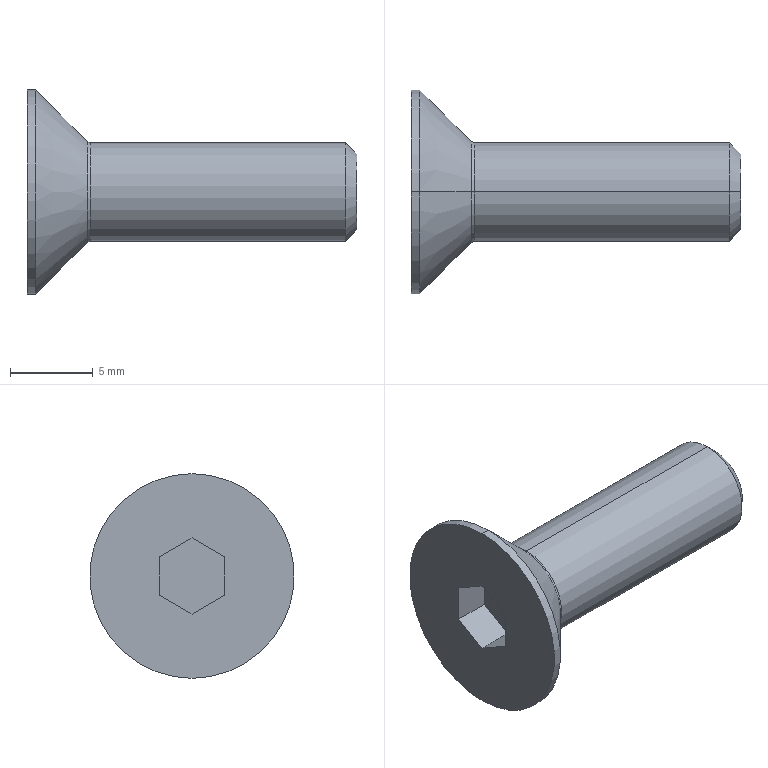Part | STEP file | 1 solid | 19 faces | box 20 x 12.399 x 12.399 mm | volume 709.68 mm3 | plane 9 | cylinder 4 | cone 4 | spline 2 | commonest cylinder face diameters 6 x2 12.399 x2
STEP:
#1=CARTESIAN_POINT('',(0.,0.,0.));
#2=DIRECTION('',(0.,0.,1.));
#3=DIRECTION('',(1.,0.,0.));
#4=AXIS2_PLACEMENT_3D('',#1,#2,#3);
#5=CARTESIAN_POINT('',(-1.52,0.,2.309));
#6=VERTEX_POINT('',#5);
#7=CARTESIAN_POINT('',(-1.52,2.,1.155));
#8=VERTEX_POINT('',#7);
#9=CARTESIAN_POINT('',(-1.52,0.,2.309));
#10=DIRECTION('',(0.,0.866,-0.5));
#11=VECTOR('',#10,1.);
#12=LINE('',#9,#11);
#13=CARTESIAN_POINT('',(-1.52,0.,0.));
#14=DIRECTION('',(-1.,0.,0.));
#15=DIRECTION('',(0.,0.,1.));
#16=AXIS2_PLACEMENT_3D('',#13,#14,#15);
#17=PLANE('',#16);
#18=CARTESIAN_POINT('',(2.309,0.));
#19=DIRECTION('',(-0.5,0.866));
#20=VECTOR('',#19,1.);
#21=LINE('',#18,#20);
#22=(GEOMETRIC_REPRESENTATION_CONTEXT(2)PARAMETRIC_REPRESENTATION_CONTEXT()REPRESENTATION_CONTEXT('',''));
#23=DEFINITIONAL_REPRESENTATION('',(#21),#22);
#24=PCURVE('',#17,#23);
#25=CARTESIAN_POINT('',(-1.52,0.,2.309));
#26=DIRECTION('',(0.,0.5,0.866));
#27=DIRECTION('',(1.,0.,0.));
#28=AXIS2_PLACEMENT_3D('',#25,#26,#27);
#29=PLANE('',#28);
#30=CARTESIAN_POINT('',(0.,0.));
#31=DIRECTION('',(0.,1.));
#32=VECTOR('',#31,1.);
#33=LINE('',#30,#32);
#34=(GEOMETRIC_REPRESENTATION_CONTEXT(2)PARAMETRIC_REPRESENTATION_CONTEXT()REPRESENTATION_CONTEXT('',''));
#35=DEFINITIONAL_REPRESENTATION('',(#33),#34);
#36=PCURVE('',#29,#35);
#37=SURFACE_CURVE('',#12,(#24,#36),.PCURVE_S1.);
#38=EDGE_CURVE('',#6,#8,#37,.T.);
#39=ORIENTED_EDGE('',*,*,#38,.T.);
#40=CARTESIAN_POINT('',(-1.52,2.,-1.155));
#41=VERTEX_POINT('',#40);
#42=CARTESIAN_POINT('',(-1.52,2.,1.155));
#43=DIRECTION('',(0.,0.,-1.));
#44=VECTOR('',#43,1.);
#45=LINE('',#42,#44);
#46=CARTESIAN_POINT('',(1.155,2.));
#47=DIRECTION('',(-1.,0.));
#48=VECTOR('',#47,1.);
#49=LINE('',#46,#48);
#50=(GEOMETRIC_REPRESENTATION_CONTEXT(2)PARAMETRIC_REPRESENTATION_CONTEXT()REPRESENTATION_CONTEXT('',''));
#51=DEFINITIONAL_REPRESENTATION('',(#49),#50);
#52=PCURVE('',#17,#51);
#53=CARTESIAN_POINT('',(-1.52,2.,1.155));
#54=DIRECTION('',(0.,1.,0.));
#55=DIRECTION('',(0.,0.,-1.));
#56=AXIS2_PLACEMENT_3D('',#53,#54,#55);
#57=PLANE('',#56);
#58=CARTESIAN_POINT('',(0.,0.));
#59=DIRECTION('',(1.,0.));
#60=VECTOR('',#59,1.);
#61=LINE('',#58,#60);
#62=(GEOMETRIC_REPRESENTATION_CONTEXT(2)PARAMETRIC_REPRESENTATION_CONTEXT()REPRESENTATION_CONTEXT('',''));
#63=DEFINITIONAL_REPRESENTATION('',(#61),#62);
#64=PCURVE('',#57,#63);
#65=SURFACE_CURVE('',#45,(#52,#64),.PCURVE_S1.);
#66=EDGE_CURVE('',#8,#41,#65,.T.);
#67=ORIENTED_EDGE('',*,*,#66,.T.);
#68=CARTESIAN_POINT('',(-1.52,0.,-2.309));
#69=VERTEX_POINT('',#68);
#70=CARTESIAN_POINT('',(-1.52,2.,-1.155));
#71=DIRECTION('',(0.,-0.866,-0.5));
#72=VECTOR('',#71,1.);
#73=LINE('',#70,#72);
#74=CARTESIAN_POINT('',(-1.155,2.));
#75=DIRECTION('',(-0.5,-0.866));
#76=VECTOR('',#75,1.);
#77=LINE('',#74,#76);
#78=(GEOMETRIC_REPRESENTATION_CONTEXT(2)PARAMETRIC_REPRESENTATION_CONTEXT()REPRESENTATION_CONTEXT('',''));
#79=DEFINITIONAL_REPRESENTATION('',(#77),#78);
#80=PCURVE('',#17,#79);
#81=CARTESIAN_POINT('',(-1.52,2.,-1.155));
#82=DIRECTION('',(0.,0.5,-0.866));
#83=DIRECTION('',(-1.,0.,0.));
#84=AXIS2_PLACEMENT_3D('',#81,#82,#83);
#85=PLANE('',#84);
#86=CARTESIAN_POINT('',(0.,0.));
#87=DIRECTION('',(0.,-1.));
#88=VECTOR('',#87,1.);
#89=LINE('',#86,#88);
#90=(GEOMETRIC_REPRESENTATION_CONTEXT(2)PARAMETRIC_REPRESENTATION_CONTEXT()REPRESENTATION_CONTEXT('',''));
#91=DEFINITIONAL_REPRESENTATION('',(#89),#90);
#92=PCURVE('',#85,#91);
#93=SURFACE_CURVE('',#73,(#80,#92),.PCURVE_S1.);
#94=EDGE_CURVE('',#41,#69,#93,.T.);
#95=ORIENTED_EDGE('',*,*,#94,.T.);
#96=CARTESIAN_POINT('',(-1.52,-2.,-1.155));
#97=VERTEX_POINT('',#96);
#98=CARTESIAN_POINT('',(-1.52,0.,-2.309));
#99=DIRECTION('',(0.,-0.866,0.5));
#100=VECTOR('',#99,1.);
#101=LINE('',#98,#100);
#102=CARTESIAN_POINT('',(-2.309,0.));
#103=DIRECTION('',(0.5,-0.866));
#104=VECTOR('',#103,1.);
#105=LINE('',#102,#104);
#106=(GEOMETRIC_REPRESENTATION_CONTEXT(2)PARAMETRIC_REPRESENTATION_CONTEXT()REPRESENTATION_CONTEXT('',''));
#107=DEFINITIONAL_REPRESENTATION('',(#105),#106);
#108=PCURVE('',#17,#107);
#109=CARTESIAN_POINT('',(-1.52,0.,-2.309));
#110=DIRECTION('',(0.,-0.5,-0.866));
#111=DIRECTION('',(0.,-0.866,0.5));
#112=AXIS2_PLACEMENT_3D('',#109,#110,#111);
#113=PLANE('',#112);
#114=CARTESIAN_POINT('',(0.,0.));
#115=DIRECTION('',(1.,0.));
#116=VECTOR('',#115,1.);
#117=LINE('',#114,#116);
#118=(GEOMETRIC_REPRESENTATION_CONTEXT(2)PARAMETRIC_REPRESENTATION_CONTEXT()REPRESENTATION_CONTEXT('',''));
#119=DEFINITIONAL_REPRESENTATION('',(#117),#118);
#120=PCURVE('',#113,#119);
#121=SURFACE_CURVE('',#101,(#108,#120),.PCURVE_S1.);
#122=EDGE_CURVE('',#69,#97,#121,.T.);
#123=ORIENTED_EDGE('',*,*,#122,.T.);
#124=CARTESIAN_POINT('',(-1.52,-2.,1.155));
#125=VERTEX_POINT('',#124);
#126=CARTESIAN_POINT('',(-1.52,-2.,-1.155));
#127=DIRECTION('',(0.,0.,1.));
#128=VECTOR('',#127,1.);
#129=LINE('',#126,#128);
#130=CARTESIAN_POINT('',(-1.155,-2.));
#131=DIRECTION('',(1.,0.));
#132=VECTOR('',#131,1.);
#133=LINE('',#130,#132);
#134=(GEOMETRIC_REPRESENTATION_CONTEXT(2)PARAMETRIC_REPRESENTATION_CONTEXT()REPRESENTATION_CONTEXT('',''));
#135=DEFINITIONAL_REPRESENTATION('',(#133),#134);
#136=PCURVE('',#17,#135);
#137=CARTESIAN_POINT('',(-1.52,-2.,-1.155));
#138=DIRECTION('',(0.,-1.,0.));
#139=DIRECTION('',(-1.,0.,0.));
#140=AXIS2_PLACEMENT_3D('',#137,#138,#139);
#141=PLANE('',#140);
#142=CARTESIAN_POINT('',(0.,0.));
#143=DIRECTION('',(0.,-1.));
#144=VECTOR('',#143,1.);
#145=LINE('',#142,#144);
#146=(GEOMETRIC_REPRESENTATION_CONTEXT(2)PARAMETRIC_REPRESENTATION_CONTEXT()REPRESENTATION_CONTEXT('',''));
#147=DEFINITIONAL_REPRESENTATION('',(#145),#146);
#148=PCURVE('',#141,#147);
#149=SURFACE_CURVE('',#129,(#136,#148),.PCURVE_S1.);
#150=EDGE_CURVE('',#97,#125,#149,.T.);
#151=ORIENTED_EDGE('',*,*,#150,.T.);
#152=CARTESIAN_POINT('',(-1.52,-2.,1.155));
#153=DIRECTION('',(0.,0.866,0.5));
#154=VECTOR('',#153,1.);
#155=LINE('',#152,#154);
#156=CARTESIAN_POINT('',(1.155,-2.));
#157=DIRECTION('',(0.5,0.866));
#158=VECTOR('',#157,1.);
#159=LINE('',#156,#158);
#160=(GEOMETRIC_REPRESENTATION_CONTEXT(2)PARAMETRIC_REPRESENTATION_CONTEXT()REPRESENTATION_CONTEXT('',''));
#161=DEFINITIONAL_REPRESENTATION('',(#159),#160);
#162=PCURVE('',#17,#161);
#163=CARTESIAN_POINT('',(-1.52,-2.,1.155));
#164=DIRECTION('',(0.,-0.5,0.866));
#165=DIRECTION('',(-1.,0.,0.));
#166=AXIS2_PLACEMENT_3D('',#163,#164,#165);
#167=PLANE('',#166);
#168=CARTESIAN_POINT('',(0.,0.));
#169=DIRECTION('',(0.,-1.));
#170=VECTOR('',#169,1.);
#171=LINE('',#168,#170);
#172=(GEOMETRIC_REPRESENTATION_CONTEXT(2)PARAMETRIC_REPRESENTATION_CONTEXT()REPRESENTATION_CONTEXT('',''));
#173=DEFINITIONAL_REPRESENTATION('',(#171),#172);
#174=PCURVE('',#167,#173);
#175=SURFACE_CURVE('',#155,(#162,#174),.PCURVE_S1.);
#176=EDGE_CURVE('',#125,#6,#175,.T.);
#177=ORIENTED_EDGE('',*,*,#176,.T.);
#178=EDGE_LOOP('',(#39,#67,#95,#123,#151,#177));
#179=FACE_BOUND('',#178,.T.);
#180=ADVANCED_FACE('',(#179),#17,.T.);
#181=CARTESIAN_POINT('',(-3.72,0.,-2.309));
#182=VERTEX_POINT('',#181);
#183=CARTESIAN_POINT('',(-1.52,0.,-2.309));
#184=DIRECTION('',(1.,0.,0.));
#185=VECTOR('',#184,1.);
#186=LINE('',#183,#185);
#187=CARTESIAN_POINT('',(0.,-2.309));
#188=DIRECTION('',(-1.,0.));
#189=VECTOR('',#188,1.);
#190=LINE('',#187,#189);
#191=(GEOMETRIC_REPRESENTATION_CONTEXT(2)PARAMETRIC_REPRESENTATION_CONTEXT()REPRESENTATION_CONTEXT('',''));
#192=DEFINITIONAL_REPRESENTATION('',(#190),#191);
#193=PCURVE('',#85,#192);
#194=CARTESIAN_POINT('',(0.,0.));
#195=DIRECTION('',(0.,-1.));
#196=VECTOR('',#195,1.);
#197=LINE('',#194,#196);
#198=(GEOMETRIC_REPRESENTATION_CONTEXT(2)PARAMETRIC_REPRESENTATION_CONTEXT()REPRESENTATION_CONTEXT('',''));
#199=DEFINITIONAL_REPRESENTATION('',(#197),#198);
#200=PCURVE('',#113,#199);
#201=SURFACE_CURVE('',#186,(#193,#200),.PCURVE_S1.);
#202=EDGE_CURVE('',#182,#69,#201,.T.);
#203=ORIENTED_EDGE('',*,*,#202,.T.);
#204=ORIENTED_EDGE('',*,*,#94,.F.);
#205=CARTESIAN_POINT('',(-3.72,2.,-1.155));
#206=VERTEX_POINT('',#205);
#207=CARTESIAN_POINT('',(-1.52,2.,-1.155));
#208=DIRECTION('',(-1.,0.,0.));
#209=VECTOR('',#208,1.);
#210=LINE('',#207,#209);
#211=CARTESIAN_POINT('',(0.,0.));
#212=DIRECTION('',(1.,0.));
#213=VECTOR('',#212,1.);
#214=LINE('',#211,#213);
#215=(GEOMETRIC_REPRESENTATION_CONTEXT(2)PARAMETRIC_REPRESENTATION_CONTEXT()REPRESENTATION_CONTEXT('',''));
#216=DEFINITIONAL_REPRESENTATION('',(#214),#215);
#217=PCURVE('',#85,#216);
#218=CARTESIAN_POINT('',(2.309,0.));
#219=DIRECTION('',(0.,1.));
#220=VECTOR('',#219,1.);
#221=LINE('',#218,#220);
#222=(GEOMETRIC_REPRESENTATION_CONTEXT(2)PARAMETRIC_REPRESENTATION_CONTEXT()REPRESENTATION_CONTEXT('',''));
#223=DEFINITIONAL_REPRESENTATION('',(#221),#222);
#224=PCURVE('',#57,#223);
#225=SURFACE_CURVE('',#210,(#217,#224),.PCURVE_S1.);
#226=EDGE_CURVE('',#41,#206,#225,.T.);
#227=ORIENTED_EDGE('',*,*,#226,.T.);
#228=CARTESIAN_POINT('',(-3.72,0.,-2.309));
#229=DIRECTION('',(0.,0.866,0.5));
#230=VECTOR('',#229,1.);
#231=LINE('',#228,#230);
#232=CARTESIAN_POINT('',(2.2,-2.309));
#233=DIRECTION('',(0.,1.));
#234=VECTOR('',#233,1.);
#235=LINE('',#232,#234);
#236=(GEOMETRIC_REPRESENTATION_CONTEXT(2)PARAMETRIC_REPRESENTATION_CONTEXT()REPRESENTATION_CONTEXT('',''));
#237=DEFINITIONAL_REPRESENTATION('',(#235),#236);
#238=PCURVE('',#85,#237);
#239=CARTESIAN_POINT('',(-3.72,0.,0.));
#240=DIRECTION('',(-1.,0.,0.));
#241=DIRECTION('',(0.,0.,1.));
#242=AXIS2_PLACEMENT_3D('',#239,#240,#241);
#243=PLANE('',#242);
#244=CARTESIAN_POINT('',(-2.309,0.));
#245=DIRECTION('',(0.5,0.866));
#246=VECTOR('',#245,1.);
#247=LINE('',#244,#246);
#248=(GEOMETRIC_REPRESENTATION_CONTEXT(2)PARAMETRIC_REPRESENTATION_CONTEXT()REPRESENTATION_CONTEXT('',''));
#249=DEFINITIONAL_REPRESENTATION('',(#247),#248);
#250=PCURVE('',#243,#249);
#251=SURFACE_CURVE('',#231,(#238,#250),.PCURVE_S1.);
#252=EDGE_CURVE('',#182,#206,#251,.T.);
#253=ORIENTED_EDGE('',*,*,#252,.F.);
#254=EDGE_LOOP('',(#203,#204,#227,#253));
#255=FACE_BOUND('',#254,.T.);
#256=ADVANCED_FACE('',(#255),#85,.F.);
#257=ORIENTED_EDGE('',*,*,#226,.F.);
#258=ORIENTED_EDGE('',*,*,#66,.F.);
#259=CARTESIAN_POINT('',(-3.72,2.,1.155));
#260=VERTEX_POINT('',#259);
#261=CARTESIAN_POINT('',(-1.52,2.,1.155));
#262=DIRECTION('',(-1.,0.,0.));
#263=VECTOR('',#262,1.);
#264=LINE('',#261,#263);
#265=CARTESIAN_POINT('',(0.,0.));
#266=DIRECTION('',(0.,1.));
#267=VECTOR('',#266,1.);
#268=LINE('',#265,#267);
#269=(GEOMETRIC_REPRESENTATION_CONTEXT(2)PARAMETRIC_REPRESENTATION_CONTEXT()REPRESENTATION_CONTEXT('',''));
#270=DEFINITIONAL_REPRESENTATION('',(#268),#269);
#271=PCURVE('',#57,#270);
#272=CARTESIAN_POINT('',(0.,2.309));
#273=DIRECTION('',(-1.,0.));
#274=VECTOR('',#273,1.);
#275=LINE('',#272,#274);
#276=(GEOMETRIC_REPRESENTATION_CONTEXT(2)PARAMETRIC_REPRESENTATION_CONTEXT()REPRESENTATION_CONTEXT('',''));
#277=DEFINITIONAL_REPRESENTATION('',(#275),#276);
#278=PCURVE('',#29,#277);
#279=SURFACE_CURVE('',#264,(#271,#278),.PCURVE_S1.);
#280=EDGE_CURVE('',#8,#260,#279,.T.);
#281=ORIENTED_EDGE('',*,*,#280,.T.);
#282=CARTESIAN_POINT('',(-3.72,2.,0.));
#283=DIRECTION('',(0.,0.,1.));
#284=VECTOR('',#283,1.);
#285=LINE('',#282,#284);
#286=CARTESIAN_POINT('',(1.155,2.2));
#287=DIRECTION('',(-1.,0.));
#288=VECTOR('',#287,1.);
#289=LINE('',#286,#288);
#290=(GEOMETRIC_REPRESENTATION_CONTEXT(2)PARAMETRIC_REPRESENTATION_CONTEXT()REPRESENTATION_CONTEXT('',''));
#291=DEFINITIONAL_REPRESENTATION('',(#289),#290);
#292=PCURVE('',#57,#291);
#293=CARTESIAN_POINT('',(0.,2.));
#294=DIRECTION('',(1.,0.));
#295=VECTOR('',#294,1.);
#296=LINE('',#293,#295);
#297=(GEOMETRIC_REPRESENTATION_CONTEXT(2)PARAMETRIC_REPRESENTATION_CONTEXT()REPRESENTATION_CONTEXT('',''));
#298=DEFINITIONAL_REPRESENTATION('',(#296),#297);
#299=PCURVE('',#243,#298);
#300=SURFACE_CURVE('',#285,(#292,#299),.PCURVE_S1.);
#301=EDGE_CURVE('',#206,#260,#300,.T.);
#302=ORIENTED_EDGE('',*,*,#301,.F.);
#303=EDGE_LOOP('',(#257,#258,#281,#302));
#304=FACE_BOUND('',#303,.T.);
#305=ADVANCED_FACE('',(#304),#57,.F.);
#306=ORIENTED_EDGE('',*,*,#280,.F.);
#307=ORIENTED_EDGE('',*,*,#38,.F.);
#308=CARTESIAN_POINT('',(-3.72,0.,2.309));
#309=VERTEX_POINT('',#308);
#310=CARTESIAN_POINT('',(-1.52,0.,2.309));
#311=DIRECTION('',(-1.,0.,0.));
#312=VECTOR('',#311,1.);
#313=LINE('',#310,#312);
#314=CARTESIAN_POINT('',(0.,0.));
#315=DIRECTION('',(-1.,0.));
#316=VECTOR('',#315,1.);
#317=LINE('',#314,#316);
#318=(GEOMETRIC_REPRESENTATION_CONTEXT(2)PARAMETRIC_REPRESENTATION_CONTEXT()REPRESENTATION_CONTEXT('',''));
#319=DEFINITIONAL_REPRESENTATION('',(#317),#318);
#320=PCURVE('',#29,#319);
#321=CARTESIAN_POINT('',(0.,-2.309));
#322=DIRECTION('',(1.,0.));
#323=VECTOR('',#322,1.);
#324=LINE('',#321,#323);
#325=(GEOMETRIC_REPRESENTATION_CONTEXT(2)PARAMETRIC_REPRESENTATION_CONTEXT()REPRESENTATION_CONTEXT('',''));
#326=DEFINITIONAL_REPRESENTATION('',(#324),#325);
#327=PCURVE('',#167,#326);
#328=SURFACE_CURVE('',#313,(#320,#327),.PCURVE_S1.);
#329=EDGE_CURVE('',#6,#309,#328,.T.);
#330=ORIENTED_EDGE('',*,*,#329,.T.);
#331=CARTESIAN_POINT('',(-3.72,2.,1.155));
#332=DIRECTION('',(0.,-0.866,0.5));
#333=VECTOR('',#332,1.);
#334=LINE('',#331,#333);
#335=CARTESIAN_POINT('',(-2.2,2.309));
#336=DIRECTION('',(0.,-1.));
#337=VECTOR('',#336,1.);
#338=LINE('',#335,#337);
#339=(GEOMETRIC_REPRESENTATION_CONTEXT(2)PARAMETRIC_REPRESENTATION_CONTEXT()REPRESENTATION_CONTEXT('',''));
#340=DEFINITIONAL_REPRESENTATION('',(#338),#339);
#341=PCURVE('',#29,#340);
#342=CARTESIAN_POINT('',(1.155,2.));
#343=DIRECTION('',(0.5,-0.866));
#344=VECTOR('',#343,1.);
#345=LINE('',#342,#344);
#346=(GEOMETRIC_REPRESENTATION_CONTEXT(2)PARAMETRIC_REPRESENTATION_CONTEXT()REPRESENTATION_CONTEXT('',''));
#347=DEFINITIONAL_REPRESENTATION('',(#345),#346);
#348=PCURVE('',#243,#347);
#349=SURFACE_CURVE('',#334,(#341,#348),.PCURVE_S1.);
#350=EDGE_CURVE('',#260,#309,#349,.T.);
#351=ORIENTED_EDGE('',*,*,#350,.F.);
#352=EDGE_LOOP('',(#306,#307,#330,#351));
#353=FACE_BOUND('',#352,.T.);
#354=ADVANCED_FACE('',(#353),#29,.F.);
#355=ORIENTED_EDGE('',*,*,#329,.F.);
#356=ORIENTED_EDGE('',*,*,#176,.F.);
#357=CARTESIAN_POINT('',(-3.72,-2.,1.155));
#358=VERTEX_POINT('',#357);
#359=CARTESIAN_POINT('',(-1.52,-2.,1.155));
#360=DIRECTION('',(-1.,0.,0.));
#361=VECTOR('',#360,1.);
#362=LINE('',#359,#361);
#363=CARTESIAN_POINT('',(0.,0.));
#364=DIRECTION('',(1.,0.));
#365=VECTOR('',#364,1.);
#366=LINE('',#363,#365);
#367=(GEOMETRIC_REPRESENTATION_CONTEXT(2)PARAMETRIC_REPRESENTATION_CONTEXT()REPRESENTATION_CONTEXT('',''));
#368=DEFINITIONAL_REPRESENTATION('',(#366),#367);
#369=PCURVE('',#167,#368);
#370=CARTESIAN_POINT('',(0.,-2.309));
#371=DIRECTION('',(1.,0.));
#372=VECTOR('',#371,1.);
#373=LINE('',#370,#372);
#374=(GEOMETRIC_REPRESENTATION_CONTEXT(2)PARAMETRIC_REPRESENTATION_CONTEXT()REPRESENTATION_CONTEXT('',''));
#375=DEFINITIONAL_REPRESENTATION('',(#373),#374);
#376=PCURVE('',#141,#375);
#377=SURFACE_CURVE('',#362,(#369,#376),.PCURVE_S1.);
#378=EDGE_CURVE('',#125,#358,#377,.T.);
#379=ORIENTED_EDGE('',*,*,#378,.T.);
#380=CARTESIAN_POINT('',(-3.72,0.,2.309));
#381=DIRECTION('',(0.,-0.866,-0.5));
#382=VECTOR('',#381,1.);
#383=LINE('',#380,#382);
#384=CARTESIAN_POINT('',(2.2,-2.309));
#385=DIRECTION('',(0.,1.));
#386=VECTOR('',#385,1.);
#387=LINE('',#384,#386);
#388=(GEOMETRIC_REPRESENTATION_CONTEXT(2)PARAMETRIC_REPRESENTATION_CONTEXT()REPRESENTATION_CONTEXT('',''));
#389=DEFINITIONAL_REPRESENTATION('',(#387),#388);
#390=PCURVE('',#167,#389);
#391=CARTESIAN_POINT('',(2.309,0.));
#392=DIRECTION('',(-0.5,-0.866));
#393=VECTOR('',#392,1.);
#394=LINE('',#391,#393);
#395=(GEOMETRIC_REPRESENTATION_CONTEXT(2)PARAMETRIC_REPRESENTATION_CONTEXT()REPRESENTATION_CONTEXT('',''));
#396=DEFINITIONAL_REPRESENTATION('',(#394),#395);
#397=PCURVE('',#243,#396);
#398=SURFACE_CURVE('',#383,(#390,#397),.PCURVE_S1.);
#399=EDGE_CURVE('',#309,#358,#398,.T.);
#400=ORIENTED_EDGE('',*,*,#399,.F.);
#401=EDGE_LOOP('',(#355,#356,#379,#400));
#402=FACE_BOUND('',#401,.T.);
#403=ADVANCED_FACE('',(#402),#167,.F.);
#404=ORIENTED_EDGE('',*,*,#378,.F.);
#405=ORIENTED_EDGE('',*,*,#150,.F.);
#406=CARTESIAN_POINT('',(-3.72,-2.,-1.155));
#407=VERTEX_POINT('',#406);
#408=CARTESIAN_POINT('',(-1.52,-2.,-1.155));
#409=DIRECTION('',(-1.,0.,0.));
#410=VECTOR('',#409,1.);
#411=LINE('',#408,#410);
#412=CARTESIAN_POINT('',(0.,0.));
#413=DIRECTION('',(1.,0.));
#414=VECTOR('',#413,1.);
#415=LINE('',#412,#414);
#416=(GEOMETRIC_REPRESENTATION_CONTEXT(2)PARAMETRIC_REPRESENTATION_CONTEXT()REPRESENTATION_CONTEXT('',''));
#417=DEFINITIONAL_REPRESENTATION('',(#415),#416);
#418=PCURVE('',#141,#417);
#419=CARTESIAN_POINT('',(2.309,0.));
#420=DIRECTION('',(0.,1.));
#421=VECTOR('',#420,1.);
#422=LINE('',#419,#421);
#423=(GEOMETRIC_REPRESENTATION_CONTEXT(2)PARAMETRIC_REPRESENTATION_CONTEXT()REPRESENTATION_CONTEXT('',''));
#424=DEFINITIONAL_REPRESENTATION('',(#422),#423);
#425=PCURVE('',#113,#424);
#426=SURFACE_CURVE('',#411,(#418,#425),.PCURVE_S1.);
#427=EDGE_CURVE('',#97,#407,#426,.T.);
#428=ORIENTED_EDGE('',*,*,#427,.T.);
#429=CARTESIAN_POINT('',(-3.72,-2.,0.));
#430=DIRECTION('',(0.,0.,-1.));
#431=VECTOR('',#430,1.);
#432=LINE('',#429,#431);
#433=CARTESIAN_POINT('',(2.2,-1.155));
#434=DIRECTION('',(0.,1.));
#435=VECTOR('',#434,1.);
#436=LINE('',#433,#435);
#437=(GEOMETRIC_REPRESENTATION_CONTEXT(2)PARAMETRIC_REPRESENTATION_CONTEXT()REPRESENTATION_CONTEXT('',''));
#438=DEFINITIONAL_REPRESENTATION('',(#436),#437);
#439=PCURVE('',#141,#438);
#440=CARTESIAN_POINT('',(0.,-2.));
#441=DIRECTION('',(-1.,0.));
#442=VECTOR('',#441,1.);
#443=LINE('',#440,#442);
#444=(GEOMETRIC_REPRESENTATION_CONTEXT(2)PARAMETRIC_REPRESENTATION_CONTEXT()REPRESENTATION_CONTEXT('',''));
#445=DEFINITIONAL_REPRESENTATION('',(#443),#444);
#446=PCURVE('',#243,#445);
#447=SURFACE_CURVE('',#432,(#439,#446),.PCURVE_S1.);
#448=EDGE_CURVE('',#358,#407,#447,.T.);
#449=ORIENTED_EDGE('',*,*,#448,.F.);
#450=EDGE_LOOP('',(#404,#405,#428,#449));
#451=FACE_BOUND('',#450,.T.);
#452=ADVANCED_FACE('',(#451),#141,.F.);
#453=ORIENTED_EDGE('',*,*,#427,.F.);
#454=ORIENTED_EDGE('',*,*,#122,.F.);
#455=ORIENTED_EDGE('',*,*,#202,.F.);
#456=CARTESIAN_POINT('',(-3.72,-2.,-1.155));
#457=DIRECTION('',(0.,0.866,-0.5));
#458=VECTOR('',#457,1.);
#459=LINE('',#456,#458);
#460=CARTESIAN_POINT('',(2.309,2.2));
#461=DIRECTION('',(-1.,0.));
#462=VECTOR('',#461,1.);
#463=LINE('',#460,#462);
#464=(GEOMETRIC_REPRESENTATION_CONTEXT(2)PARAMETRIC_REPRESENTATION_CONTEXT()REPRESENTATION_CONTEXT('',''));
#465=DEFINITIONAL_REPRESENTATION('',(#463),#464);
#466=PCURVE('',#113,#465);
#467=CARTESIAN_POINT('',(-1.155,-2.));
#468=DIRECTION('',(-0.5,0.866));
#469=VECTOR('',#468,1.);
#470=LINE('',#467,#469);
#471=(GEOMETRIC_REPRESENTATION_CONTEXT(2)PARAMETRIC_REPRESENTATION_CONTEXT()REPRESENTATION_CONTEXT('',''));
#472=DEFINITIONAL_REPRESENTATION('',(#470),#471);
#473=PCURVE('',#243,#472);
#474=SURFACE_CURVE('',#459,(#466,#473),.PCURVE_S1.);
#475=EDGE_CURVE('',#407,#182,#474,.T.);
#476=ORIENTED_EDGE('',*,*,#475,.F.);
#477=EDGE_LOOP('',(#453,#454,#455,#476));
#478=FACE_BOUND('',#477,.T.);
#479=ADVANCED_FACE('',(#478),#113,.F.);
#480=ORIENTED_EDGE('',*,*,#448,.T.);
#481=ORIENTED_EDGE('',*,*,#475,.T.);
#482=ORIENTED_EDGE('',*,*,#252,.T.);
#483=ORIENTED_EDGE('',*,*,#301,.T.);
#484=ORIENTED_EDGE('',*,*,#350,.T.);
#485=ORIENTED_EDGE('',*,*,#399,.T.);
#486=EDGE_LOOP('',(#480,#481,#482,#483,#484,#485));
#487=FACE_BOUND('',#486,.T.);
#488=CARTESIAN_POINT('',(-3.72,0.,6.2));
#489=VERTEX_POINT('',#488);
#490=CARTESIAN_POINT('',(-3.72,0.,-6.2));
#491=VERTEX_POINT('',#490);
#492=CARTESIAN_POINT('',(-3.72,0.,0.));
#493=DIRECTION('',(1.,0.,0.));
#494=DIRECTION('',(0.,0.,1.));
#495=AXIS2_PLACEMENT_3D('',#492,#493,#494);
#496=CIRCLE('',#495,6.2);
#497=CARTESIAN_POINT('',(6.2,0.));
#498=CARTESIAN_POINT('',(6.2,-10.738));
#499=CARTESIAN_POINT('',(-3.1,-5.369));
#500=CARTESIAN_POINT('',(-12.399,0.));
#501=CARTESIAN_POINT('',(-3.1,5.369));
#502=CARTESIAN_POINT('',(6.2,10.738));
#503=CARTESIAN_POINT('',(6.2,0.));
#504=(BOUNDED_CURVE()B_SPLINE_CURVE(2,(#497,#498,#499,#500,#501,#502,#503),.UNSPECIFIED.,.T.,.F.)B_SPLINE_CURVE_WITH_KNOTS((1,2,2,2,2,1),(-2.094,0.,2.094,4.189,6.283,8.378),.UNSPECIFIED.)CURVE()GEOMETRIC_REPRESENTATION_ITEM()RATIONAL_B_SPLINE_CURVE((1.,0.5,1.,0.5,1.,0.5,1.))REPRESENTATION_ITEM(''));
#505=(GEOMETRIC_REPRESENTATION_CONTEXT(2)PARAMETRIC_REPRESENTATION_CONTEXT()REPRESENTATION_CONTEXT('',''));
#506=DEFINITIONAL_REPRESENTATION('',(#504),#505);
#507=PCURVE('',#243,#506);
#508=CARTESIAN_POINT('',(16.28,0.,0.));
#509=DIRECTION('',(-1.,0.,0.));
#510=DIRECTION('',(0.,0.,1.));
#511=AXIS2_PLACEMENT_3D('',#508,#509,#510);
#512=CYLINDRICAL_SURFACE('',#511,6.2);
#513=CARTESIAN_POINT('',(6.283,20.));
#514=DIRECTION('',(-1.,0.));
#515=VECTOR('',#514,1.);
#516=LINE('',#513,#515);
#517=(GEOMETRIC_REPRESENTATION_CONTEXT(2)PARAMETRIC_REPRESENTATION_CONTEXT()REPRESENTATION_CONTEXT('',''));
#518=DEFINITIONAL_REPRESENTATION('',(#516),#517);
#519=PCURVE('',#512,#518);
#520=SURFACE_CURVE('',#496,(#507,#519),.PCURVE_S1.);
#521=EDGE_CURVE('',#489,#491,#520,.T.);
#522=ORIENTED_EDGE('',*,*,#521,.F.);
#523=CARTESIAN_POINT('',(-3.72,0.,0.));
#524=DIRECTION('',(1.,0.,0.));
#525=DIRECTION('',(0.,0.,1.));
#526=AXIS2_PLACEMENT_3D('',#523,#524,#525);
#527=CIRCLE('',#526,6.2);
#528=CARTESIAN_POINT('',(6.2,0.));
#529=CARTESIAN_POINT('',(6.2,-10.738));
#530=CARTESIAN_POINT('',(-3.1,-5.369));
#531=CARTESIAN_POINT('',(-12.399,0.));
#532=CARTESIAN_POINT('',(-3.1,5.369));
#533=CARTESIAN_POINT('',(6.2,10.738));
#534=CARTESIAN_POINT('',(6.2,0.));
#535=(BOUNDED_CURVE()B_SPLINE_CURVE(2,(#528,#529,#530,#531,#532,#533,#534),.UNSPECIFIED.,.T.,.F.)B_SPLINE_CURVE_WITH_KNOTS((1,2,2,2,2,1),(-2.094,0.,2.094,4.189,6.283,8.378),.UNSPECIFIED.)CURVE()GEOMETRIC_REPRESENTATION_ITEM()RATIONAL_B_SPLINE_CURVE((1.,0.5,1.,0.5,1.,0.5,1.))REPRESENTATION_ITEM(''));
#536=(GEOMETRIC_REPRESENTATION_CONTEXT(2)PARAMETRIC_REPRESENTATION_CONTEXT()REPRESENTATION_CONTEXT('',''));
#537=DEFINITIONAL_REPRESENTATION('',(#535),#536);
#538=PCURVE('',#243,#537);
#539=CARTESIAN_POINT('',(16.28,0.,0.));
#540=DIRECTION('',(-1.,0.,0.));
#541=DIRECTION('',(0.,0.,1.));
#542=AXIS2_PLACEMENT_3D('',#539,#540,#541);
#543=CYLINDRICAL_SURFACE('',#542,6.2);
#544=CARTESIAN_POINT('',(6.283,20.));
#545=DIRECTION('',(-1.,0.));
#546=VECTOR('',#545,1.);
#547=LINE('',#544,#546);
#548=(GEOMETRIC_REPRESENTATION_CONTEXT(2)PARAMETRIC_REPRESENTATION_CONTEXT()REPRESENTATION_CONTEXT('',''));
#549=DEFINITIONAL_REPRESENTATION('',(#547),#548);
#550=PCURVE('',#543,#549);
#551=SURFACE_CURVE('',#527,(#538,#550),.PCURVE_S1.);
#552=EDGE_CURVE('',#491,#489,#551,.T.);
#553=ORIENTED_EDGE('',*,*,#552,.F.);
#554=EDGE_LOOP('',(#522,#553));
#555=FACE_BOUND('',#554,.T.);
#556=ADVANCED_FACE('',(#487,#555),#243,.T.);
#557=CARTESIAN_POINT('',(-3.2,0.,-6.2));
#558=VERTEX_POINT('',#557);
#559=CARTESIAN_POINT('',(16.28,0.,-6.2));
#560=DIRECTION('',(-1.,0.,0.));
#561=VECTOR('',#560,1.);
#562=LINE('',#559,#561);
#563=CARTESIAN_POINT('',(3.142,0.));
#564=DIRECTION('',(0.,1.));
#565=VECTOR('',#564,1.);
#566=LINE('',#563,#565);
#567=(GEOMETRIC_REPRESENTATION_CONTEXT(2)PARAMETRIC_REPRESENTATION_CONTEXT()REPRESENTATION_CONTEXT('',''));
#568=DEFINITIONAL_REPRESENTATION('',(#566),#567);
#569=PCURVE('',#512,#568);
#570=CARTESIAN_POINT('',(3.142,0.));
#571=DIRECTION('',(0.,1.));
#572=VECTOR('',#571,1.);
#573=LINE('',#570,#572);
#574=(GEOMETRIC_REPRESENTATION_CONTEXT(2)PARAMETRIC_REPRESENTATION_CONTEXT()REPRESENTATION_CONTEXT('',''));
#575=DEFINITIONAL_REPRESENTATION('',(#573),#574);
#576=PCURVE('',#543,#575);
#577=SURFACE_CURVE('',#562,(#569,#576),.PCURVE_S1.);
#578=EDGE_CURVE('',#558,#491,#577,.T.);
#579=ORIENTED_EDGE('',*,*,#578,.F.);
#580=CARTESIAN_POINT('',(-3.2,0.,6.2));
#581=VERTEX_POINT('',#580);
#582=CARTESIAN_POINT('',(-3.2,0.,0.));
#583=DIRECTION('',(1.,0.,0.));
#584=DIRECTION('',(0.,0.,1.));
#585=AXIS2_PLACEMENT_3D('',#582,#583,#584);
#586=CIRCLE('',#585,6.2);
#587=CARTESIAN_POINT('',(6.283,19.48));
#588=DIRECTION('',(-1.,0.));
#589=VECTOR('',#588,1.);
#590=LINE('',#587,#589);
#591=(GEOMETRIC_REPRESENTATION_CONTEXT(2)PARAMETRIC_REPRESENTATION_CONTEXT()REPRESENTATION_CONTEXT('',''));
#592=DEFINITIONAL_REPRESENTATION('',(#590),#591);
#593=PCURVE('',#512,#592);
#594=CARTESIAN_POINT('',(-3.2,0.,0.));
#595=DIRECTION('',(-1.,0.,0.));
#596=DIRECTION('',(0.,0.,1.));
#597=AXIS2_PLACEMENT_3D('',#594,#595,#596);
#598=CONICAL_SURFACE('',#597,6.2,0.7854);
#599=CARTESIAN_POINT('',(6.283,0.));
#600=DIRECTION('',(-1.,0.));
#601=VECTOR('',#600,1.);
#602=LINE('',#599,#601);
#603=(GEOMETRIC_REPRESENTATION_CONTEXT(2)PARAMETRIC_REPRESENTATION_CONTEXT()REPRESENTATION_CONTEXT('',''));
#604=DEFINITIONAL_REPRESENTATION('',(#602),#603);
#605=PCURVE('',#598,#604);
#606=SURFACE_CURVE('',#586,(#593,#605),.PCURVE_S1.);
#607=EDGE_CURVE('',#581,#558,#606,.T.);
#608=ORIENTED_EDGE('',*,*,#607,.F.);
#609=CARTESIAN_POINT('',(16.28,0.,6.2));
#610=DIRECTION('',(-1.,0.,0.));
#611=VECTOR('',#610,1.);
#612=LINE('',#609,#611);
#613=CARTESIAN_POINT('',(6.283,0.));
#614=DIRECTION('',(0.,1.));
#615=VECTOR('',#614,1.);
#616=LINE('',#613,#615);
#617=(GEOMETRIC_REPRESENTATION_CONTEXT(2)PARAMETRIC_REPRESENTATION_CONTEXT()REPRESENTATION_CONTEXT('',''));
#618=DEFINITIONAL_REPRESENTATION('',(#616),#617);
#619=PCURVE('',#512,#618);
#620=CARTESIAN_POINT('',(0.,0.));
#621=DIRECTION('',(0.,1.));
#622=VECTOR('',#621,1.);
#623=LINE('',#620,#622);
#624=(GEOMETRIC_REPRESENTATION_CONTEXT(2)PARAMETRIC_REPRESENTATION_CONTEXT()REPRESENTATION_CONTEXT('',''));
#625=DEFINITIONAL_REPRESENTATION('',(#623),#624);
#626=PCURVE('',#543,#625);
#627=SURFACE_CURVE('',#612,(#619,#626),.PCURVE_S1.);
#628=EDGE_CURVE('',#581,#489,#627,.T.);
#629=ORIENTED_EDGE('',*,*,#628,.T.);
#630=ORIENTED_EDGE('',*,*,#521,.T.);
#631=EDGE_LOOP('',(#579,#608,#629,#630));
#632=FACE_BOUND('',#631,.T.);
#633=ADVANCED_FACE('',(#632),#512,.T.);
#634=CARTESIAN_POINT('',(16.28,0.,2.3));
#635=VERTEX_POINT('',#634);
#636=CARTESIAN_POINT('',(16.28,0.,-2.3));
#637=VERTEX_POINT('',#636);
#638=CARTESIAN_POINT('',(16.28,0.,0.));
#639=DIRECTION('',(-1.,0.,0.));
#640=DIRECTION('',(0.,0.,1.));
#641=AXIS2_PLACEMENT_3D('',#638,#639,#640);
#642=CIRCLE('',#641,2.3);
#643=CARTESIAN_POINT('',(16.28,3.,0.));
#644=DIRECTION('',(1.,0.,0.));
#645=DIRECTION('',(0.,1.,0.));
#646=AXIS2_PLACEMENT_3D('',#643,#644,#645);
#647=PLANE('',#646);
#648=CARTESIAN_POINT('',(-3.,2.3));
#649=CARTESIAN_POINT('',(0.9837,2.3));
#650=CARTESIAN_POINT('',(-1.008,-1.15));
#651=CARTESIAN_POINT('',(-3.,-4.6));
#652=CARTESIAN_POINT('',(-4.992,-1.15));
#653=CARTESIAN_POINT('',(-6.984,2.3));
#654=CARTESIAN_POINT('',(-3.,2.3));
#655=(BOUNDED_CURVE()B_SPLINE_CURVE(2,(#648,#649,#650,#651,#652,#653,#654),.UNSPECIFIED.,.T.,.F.)B_SPLINE_CURVE_WITH_KNOTS((1,2,2,2,2,1),(-2.094,0.,2.094,4.189,6.283,8.378),.UNSPECIFIED.)CURVE()GEOMETRIC_REPRESENTATION_ITEM()RATIONAL_B_SPLINE_CURVE((1.,0.5,1.,0.5,1.,0.5,1.))REPRESENTATION_ITEM(''));
#656=(GEOMETRIC_REPRESENTATION_CONTEXT(2)PARAMETRIC_REPRESENTATION_CONTEXT()REPRESENTATION_CONTEXT('',''));
#657=DEFINITIONAL_REPRESENTATION('',(#655),#656);
#658=PCURVE('',#647,#657);
#659=CARTESIAN_POINT('',(15.58,0.,0.));
#660=DIRECTION('',(-1.,0.,0.));
#661=DIRECTION('',(0.,0.,1.));
#662=AXIS2_PLACEMENT_3D('',#659,#660,#661);
#663=CONICAL_SURFACE('',#662,3.,0.7854);
#664=CARTESIAN_POINT('',(0.,-0.7));
#665=DIRECTION('',(1.,0.));
#666=VECTOR('',#665,1.);
#667=LINE('',#664,#666);
#668=(GEOMETRIC_REPRESENTATION_CONTEXT(2)PARAMETRIC_REPRESENTATION_CONTEXT()REPRESENTATION_CONTEXT('',''));
#669=DEFINITIONAL_REPRESENTATION('',(#667),#668);
#670=PCURVE('',#663,#669);
#671=SURFACE_CURVE('',#642,(#658,#670),.PCURVE_S1.);
#672=EDGE_CURVE('',#635,#637,#671,.T.);
#673=ORIENTED_EDGE('',*,*,#672,.F.);
#674=CARTESIAN_POINT('',(16.28,0.,0.));
#675=DIRECTION('',(-1.,0.,0.));
#676=DIRECTION('',(0.,0.,1.));
#677=AXIS2_PLACEMENT_3D('',#674,#675,#676);
#678=CIRCLE('',#677,2.3);
#679=CARTESIAN_POINT('',(-3.,2.3));
#680=CARTESIAN_POINT('',(0.9837,2.3));
#681=CARTESIAN_POINT('',(-1.008,-1.15));
#682=CARTESIAN_POINT('',(-3.,-4.6));
#683=CARTESIAN_POINT('',(-4.992,-1.15));
#684=CARTESIAN_POINT('',(-6.984,2.3));
#685=CARTESIAN_POINT('',(-3.,2.3));
#686=(BOUNDED_CURVE()B_SPLINE_CURVE(2,(#679,#680,#681,#682,#683,#684,#685),.UNSPECIFIED.,.T.,.F.)B_SPLINE_CURVE_WITH_KNOTS((1,2,2,2,2,1),(-2.094,0.,2.094,4.189,6.283,8.378),.UNSPECIFIED.)CURVE()GEOMETRIC_REPRESENTATION_ITEM()RATIONAL_B_SPLINE_CURVE((1.,0.5,1.,0.5,1.,0.5,1.))REPRESENTATION_ITEM(''));
#687=(GEOMETRIC_REPRESENTATION_CONTEXT(2)PARAMETRIC_REPRESENTATION_CONTEXT()REPRESENTATION_CONTEXT('',''));
#688=DEFINITIONAL_REPRESENTATION('',(#686),#687);
#689=PCURVE('',#647,#688);
#690=CARTESIAN_POINT('',(15.58,0.,0.));
#691=DIRECTION('',(-1.,0.,0.));
#692=DIRECTION('',(0.,0.,1.));
#693=AXIS2_PLACEMENT_3D('',#690,#691,#692);
#694=CONICAL_SURFACE('',#693,3.,0.7854);
#695=CARTESIAN_POINT('',(0.,-0.7));
#696=DIRECTION('',(1.,0.));
#697=VECTOR('',#696,1.);
#698=LINE('',#695,#697);
#699=(GEOMETRIC_REPRESENTATION_CONTEXT(2)PARAMETRIC_REPRESENTATION_CONTEXT()REPRESENTATION_CONTEXT('',''));
#700=DEFINITIONAL_REPRESENTATION('',(#698),#699);
#701=PCURVE('',#694,#700);
#702=SURFACE_CURVE('',#678,(#689,#701),.PCURVE_S1.);
#703=EDGE_CURVE('',#637,#635,#702,.T.);
#704=ORIENTED_EDGE('',*,*,#703,.F.);
#705=EDGE_LOOP('',(#673,#704));
#706=FACE_BOUND('',#705,.T.);
#707=ADVANCED_FACE('',(#706),#647,.T.);
#708=CARTESIAN_POINT('',(-0.07322,0.,-3.073));
#709=VERTEX_POINT('',#708);
#710=CARTESIAN_POINT('',(-3.2,0.,-6.2));
#711=DIRECTION('',(-0.7071,0.,-0.7071));
#712=VECTOR('',#711,1.);
#713=LINE('',#710,#712);
#714=CARTESIAN_POINT('',(3.142,0.));
#715=DIRECTION('',(0.,1.));
#716=VECTOR('',#715,1.);
#717=LINE('',#714,#716);
#718=(GEOMETRIC_REPRESENTATION_CONTEXT(2)PARAMETRIC_REPRESENTATION_CONTEXT()REPRESENTATION_CONTEXT('',''));
#719=DEFINITIONAL_REPRESENTATION('',(#717),#718);
#720=PCURVE('',#598,#719);
#721=CARTESIAN_POINT('',(-3.2,0.,0.));
#722=DIRECTION('',(-1.,0.,0.));
#723=DIRECTION('',(0.,0.,1.));
#724=AXIS2_PLACEMENT_3D('',#721,#722,#723);
#725=CONICAL_SURFACE('',#724,6.2,0.7854);
#726=CARTESIAN_POINT('',(3.142,0.));
#727=DIRECTION('',(0.,1.));
#728=VECTOR('',#727,1.);
#729=LINE('',#726,#728);
#730=(GEOMETRIC_REPRESENTATION_CONTEXT(2)PARAMETRIC_REPRESENTATION_CONTEXT()REPRESENTATION_CONTEXT('',''));
#731=DEFINITIONAL_REPRESENTATION('',(#729),#730);
#732=PCURVE('',#725,#731);
#733=SURFACE_CURVE('',#713,(#720,#732),.PCURVE_S1.);
#734=EDGE_CURVE('',#709,#558,#733,.T.);
#735=ORIENTED_EDGE('',*,*,#734,.F.);
#736=CARTESIAN_POINT('',(-0.07322,0.,3.073));
#737=VERTEX_POINT('',#736);
#738=CARTESIAN_POINT('',(-0.07322,0.,0.));
#739=DIRECTION('',(-1.,0.,0.));
#740=DIRECTION('',(0.,0.,1.));
#741=AXIS2_PLACEMENT_3D('',#738,#739,#740);
#742=CIRCLE('',#741,3.073);
#743=CARTESIAN_POINT('',(0.,-3.126));
#744=DIRECTION('',(1.,0.));
#745=VECTOR('',#744,1.);
#746=LINE('',#743,#745);
#747=(GEOMETRIC_REPRESENTATION_CONTEXT(2)PARAMETRIC_REPRESENTATION_CONTEXT()REPRESENTATION_CONTEXT('',''));
#748=DEFINITIONAL_REPRESENTATION('',(#746),#747);
#749=PCURVE('',#598,#748);
#750=CARTESIAN_POINT('',(0.1036,0.,-3.));
#751=CARTESIAN_POINT('',(0.1036,-6.,-3.));
#752=CARTESIAN_POINT('',(0.1036,-6.,3.));
#753=CARTESIAN_POINT('',(0.1036,0.,3.));
#754=CARTESIAN_POINT('',(0.03636,0.,-3.));
#755=CARTESIAN_POINT('',(0.03636,-6.,-3.));
#756=CARTESIAN_POINT('',(0.03636,-6.,3.));
#757=CARTESIAN_POINT('',(0.03636,0.,3.));
#758=CARTESIAN_POINT('',(-0.02571,0.,-3.026));
#759=CARTESIAN_POINT('',(-0.02571,-6.051,-3.026));
#760=CARTESIAN_POINT('',(-0.02571,-6.051,3.026));
#761=CARTESIAN_POINT('',(-0.02571,0.,3.026));
#762=CARTESIAN_POINT('',(-0.07322,0.,-3.073));
#763=CARTESIAN_POINT('',(-0.07322,-6.146,-3.073));
#764=CARTESIAN_POINT('',(-0.07322,-6.146,3.073));
#765=CARTESIAN_POINT('',(-0.07322,0.,3.073));
#766=(BOUNDED_SURFACE()B_SPLINE_SURFACE(3,3,((#750,#751,#752,#753),(#754,#755,#756,#757),(#758,#759,#760,#761),(#762,#763,#764,#765)),.UNSPECIFIED.,.F.,.F.,.F.)B_SPLINE_SURFACE_WITH_KNOTS((4,4),(4,4),(0.,1.),(0.,1.),.PIECEWISE_BEZIER_KNOTS.)GEOMETRIC_REPRESENTATION_ITEM()RATIONAL_B_SPLINE_SURFACE(((1.,0.3333,0.3333,1.),(0.9493,0.3164,0.3164,0.9493),(0.9493,0.3164,0.3164,0.9493),(1.,0.3333,0.3333,1.)))REPRESENTATION_ITEM('')SURFACE());
#767=CARTESIAN_POINT('',(1.,0.));
#768=CARTESIAN_POINT('',(1.,0.02375));
#769=CARTESIAN_POINT('',(1.,0.06805));
#770=CARTESIAN_POINT('',(1.,0.1267));
#771=CARTESIAN_POINT('',(1.,0.1794));
#772=CARTESIAN_POINT('',(1.,0.2276));
#773=CARTESIAN_POINT('',(1.,0.2721));
#774=CARTESIAN_POINT('',(1.,0.3139));
#775=CARTESIAN_POINT('',(1.,0.3535));
#776=CARTESIAN_POINT('',(1.,0.3914));
#777=CARTESIAN_POINT('',(1.,0.4282));
#778=CARTESIAN_POINT('',(1.,0.4643));
#779=CARTESIAN_POINT('',(1.,0.5));
#780=CARTESIAN_POINT('',(1.,0.5357));
#781=CARTESIAN_POINT('',(1.,0.5718));
#782=CARTESIAN_POINT('',(1.,0.6086));
#783=CARTESIAN_POINT('',(1.,0.6465));
#784=CARTESIAN_POINT('',(1.,0.6861));
#785=CARTESIAN_POINT('',(1.,0.7279));
#786=CARTESIAN_POINT('',(1.,0.7724));
#787=CARTESIAN_POINT('',(1.,0.8206));
#788=CARTESIAN_POINT('',(1.,0.8733));
#789=CARTESIAN_POINT('',(1.,0.9319));
#790=CARTESIAN_POINT('',(1.,0.9763));
#791=CARTESIAN_POINT('',(1.,1.));
#792=B_SPLINE_CURVE_WITH_KNOTS('',3,(#767,#768,#769,#770,#771,#772,#773,#774,#775,#776,#777,#778,#779,#780,#781,#782,#783,#784,#785,#786,#787,#788,#789,#790,#791),.UNSPECIFIED.,.F.,.F.,(4,1,1,1,1,1,1,1,1,1,1,1,1,1,1,1,1,1,1,1,1,1,4),(3.142,3.284,3.427,3.57,3.713,3.856,3.998,4.141,4.284,4.427,4.57,4.712,4.855,4.998,5.141,5.284,5.426,5.569,5.712,5.855,5.998,6.14,6.283),.QUASI_UNIFORM_KNOTS.);
#793=(GEOMETRIC_REPRESENTATION_CONTEXT(2)PARAMETRIC_REPRESENTATION_CONTEXT()REPRESENTATION_CONTEXT('',''));
#794=DEFINITIONAL_REPRESENTATION('',(#792),#793);
#795=PCURVE('',#766,#794);
#796=SURFACE_CURVE('',#742,(#749,#795),.PCURVE_S1.);
#797=EDGE_CURVE('',#709,#737,#796,.T.);
#798=ORIENTED_EDGE('',*,*,#797,.T.);
#799=CARTESIAN_POINT('',(-3.2,0.,6.2));
#800=DIRECTION('',(-0.7071,0.,0.7071));
#801=VECTOR('',#800,1.);
#802=LINE('',#799,#801);
#803=CARTESIAN_POINT('',(6.283,0.));
#804=DIRECTION('',(0.,1.));
#805=VECTOR('',#804,1.);
#806=LINE('',#803,#805);
#807=(GEOMETRIC_REPRESENTATION_CONTEXT(2)PARAMETRIC_REPRESENTATION_CONTEXT()REPRESENTATION_CONTEXT('',''));
#808=DEFINITIONAL_REPRESENTATION('',(#806),#807);
#809=PCURVE('',#598,#808);
#810=CARTESIAN_POINT('',(0.,0.));
#811=DIRECTION('',(0.,1.));
#812=VECTOR('',#811,1.);
#813=LINE('',#810,#812);
#814=(GEOMETRIC_REPRESENTATION_CONTEXT(2)PARAMETRIC_REPRESENTATION_CONTEXT()REPRESENTATION_CONTEXT('',''));
#815=DEFINITIONAL_REPRESENTATION('',(#813),#814);
#816=PCURVE('',#725,#815);
#817=SURFACE_CURVE('',#802,(#809,#816),.PCURVE_S1.);
#818=EDGE_CURVE('',#737,#581,#817,.T.);
#819=ORIENTED_EDGE('',*,*,#818,.T.);
#820=ORIENTED_EDGE('',*,*,#607,.T.);
#821=EDGE_LOOP('',(#735,#798,#819,#820));
#822=FACE_BOUND('',#821,.T.);
#823=ADVANCED_FACE('',(#822),#598,.T.);
#824=CARTESIAN_POINT('',(15.58,0.,-3.));
#825=VERTEX_POINT('',#824);
#826=CARTESIAN_POINT('',(15.58,0.,-3.));
#827=DIRECTION('',(-0.7071,0.,-0.7071));
#828=VECTOR('',#827,1.);
#829=LINE('',#826,#828);
#830=CARTESIAN_POINT('',(3.142,0.));
#831=DIRECTION('',(0.,1.));
#832=VECTOR('',#831,1.);
#833=LINE('',#830,#832);
#834=(GEOMETRIC_REPRESENTATION_CONTEXT(2)PARAMETRIC_REPRESENTATION_CONTEXT()REPRESENTATION_CONTEXT('',''));
#835=DEFINITIONAL_REPRESENTATION('',(#833),#834);
#836=PCURVE('',#694,#835);
#837=CARTESIAN_POINT('',(3.142,0.));
#838=DIRECTION('',(0.,1.));
#839=VECTOR('',#838,1.);
#840=LINE('',#837,#839);
#841=(GEOMETRIC_REPRESENTATION_CONTEXT(2)PARAMETRIC_REPRESENTATION_CONTEXT()REPRESENTATION_CONTEXT('',''));
#842=DEFINITIONAL_REPRESENTATION('',(#840),#841);
#843=PCURVE('',#663,#842);
#844=SURFACE_CURVE('',#829,(#836,#843),.PCURVE_S1.);
#845=EDGE_CURVE('',#637,#825,#844,.T.);
#846=ORIENTED_EDGE('',*,*,#845,.F.);
#847=ORIENTED_EDGE('',*,*,#703,.T.);
#848=CARTESIAN_POINT('',(15.58,0.,3.));
#849=VERTEX_POINT('',#848);
#850=CARTESIAN_POINT('',(15.58,0.,3.));
#851=DIRECTION('',(-0.7071,0.,0.7071));
#852=VECTOR('',#851,1.);
#853=LINE('',#850,#852);
#854=CARTESIAN_POINT('',(6.283,0.));
#855=DIRECTION('',(0.,1.));
#856=VECTOR('',#855,1.);
#857=LINE('',#854,#856);
#858=(GEOMETRIC_REPRESENTATION_CONTEXT(2)PARAMETRIC_REPRESENTATION_CONTEXT()REPRESENTATION_CONTEXT('',''));
#859=DEFINITIONAL_REPRESENTATION('',(#857),#858);
#860=PCURVE('',#694,#859);
#861=CARTESIAN_POINT('',(0.,0.));
#862=DIRECTION('',(0.,1.));
#863=VECTOR('',#862,1.);
#864=LINE('',#861,#863);
#865=(GEOMETRIC_REPRESENTATION_CONTEXT(2)PARAMETRIC_REPRESENTATION_CONTEXT()REPRESENTATION_CONTEXT('',''));
#866=DEFINITIONAL_REPRESENTATION('',(#864),#865);
#867=PCURVE('',#663,#866);
#868=SURFACE_CURVE('',#853,(#860,#867),.PCURVE_S1.);
#869=EDGE_CURVE('',#635,#849,#868,.T.);
#870=ORIENTED_EDGE('',*,*,#869,.T.);
#871=CARTESIAN_POINT('',(15.58,0.,0.));
#872=DIRECTION('',(-1.,0.,0.));
#873=DIRECTION('',(0.,0.,1.));
#874=AXIS2_PLACEMENT_3D('',#871,#872,#873);
#875=CIRCLE('',#874,3.);
#876=CARTESIAN_POINT('',(0.,0.));
#877=DIRECTION('',(1.,0.));
#878=VECTOR('',#877,1.);
#879=LINE('',#876,#878);
#880=(GEOMETRIC_REPRESENTATION_CONTEXT(2)PARAMETRIC_REPRESENTATION_CONTEXT()REPRESENTATION_CONTEXT('',''));
#881=DEFINITIONAL_REPRESENTATION('',(#879),#880);
#882=PCURVE('',#694,#881);
#883=CARTESIAN_POINT('',(16.28,0.,0.));
#884=DIRECTION('',(-1.,0.,0.));
#885=DIRECTION('',(0.,0.,1.));
#886=AXIS2_PLACEMENT_3D('',#883,#884,#885);
#887=CYLINDRICAL_SURFACE('',#886,3.);
#888=CARTESIAN_POINT('',(0.,0.7));
#889=DIRECTION('',(1.,0.));
#890=VECTOR('',#889,1.);
#891=LINE('',#888,#890);
#892=(GEOMETRIC_REPRESENTATION_CONTEXT(2)PARAMETRIC_REPRESENTATION_CONTEXT()REPRESENTATION_CONTEXT('',''));
#893=DEFINITIONAL_REPRESENTATION('',(#891),#892);
#894=PCURVE('',#887,#893);
#895=SURFACE_CURVE('',#875,(#882,#894),.PCURVE_S1.);
#896=EDGE_CURVE('',#825,#849,#895,.T.);
#897=ORIENTED_EDGE('',*,*,#896,.F.);
#898=EDGE_LOOP('',(#846,#847,#870,#897));
#899=FACE_BOUND('',#898,.T.);
#900=ADVANCED_FACE('',(#899),#694,.T.);
#901=ORIENTED_EDGE('',*,*,#797,.T.);
#902=CARTESIAN_POINT('',(0.1036,0.,3.));
#903=VERTEX_POINT('',#902);
#904=CARTESIAN_POINT('',(0.1036,0.,3.25));
#905=DIRECTION('',(0.,1.,0.));
#906=DIRECTION('',(0.,0.,1.));
#907=AXIS2_PLACEMENT_3D('',#904,#905,#906);
#908=CIRCLE('',#907,0.25);
#909=CARTESIAN_POINT('',(0.,1.));
#910=CARTESIAN_POINT('',(0.01555,1.));
#911=CARTESIAN_POINT('',(0.04653,1.));
#912=CARTESIAN_POINT('',(0.09271,1.));
#913=CARTESIAN_POINT('',(0.1386,1.));
#914=CARTESIAN_POINT('',(0.1843,1.));
#915=CARTESIAN_POINT('',(0.2298,1.));
#916=CARTESIAN_POINT('',(0.2751,1.));
#917=CARTESIAN_POINT('',(0.3202,1.));
#918=CARTESIAN_POINT('',(0.3653,1.));
#919=CARTESIAN_POINT('',(0.4102,1.));
#920=CARTESIAN_POINT('',(0.4551,1.));
#921=CARTESIAN_POINT('',(0.5,1.));
#922=CARTESIAN_POINT('',(0.5449,1.));
#923=CARTESIAN_POINT('',(0.5898,1.));
#924=CARTESIAN_POINT('',(0.6347,1.));
#925=CARTESIAN_POINT('',(0.6798,1.));
#926=CARTESIAN_POINT('',(0.7249,1.));
#927=CARTESIAN_POINT('',(0.7702,1.));
#928=CARTESIAN_POINT('',(0.8157,1.));
#929=CARTESIAN_POINT('',(0.8614,1.));
#930=CARTESIAN_POINT('',(0.9073,1.));
#931=CARTESIAN_POINT('',(0.9535,1.));
#932=CARTESIAN_POINT('',(0.9845,1.));
#933=CARTESIAN_POINT('',(1.,1.));
#934=B_SPLINE_CURVE_WITH_KNOTS('',3,(#909,#910,#911,#912,#913,#914,#915,#916,#917,#918,#919,#920,#921,#922,#923,#924,#925,#926,#927,#928,#929,#930,#931,#932,#933),.UNSPECIFIED.,.F.,.F.,(4,1,1,1,1,1,1,1,1,1,1,1,1,1,1,1,1,1,1,1,1,1,4),(3.142,3.177,3.213,3.249,3.284,3.32,3.356,3.391,3.427,3.463,3.499,3.534,3.57,3.606,3.641,3.677,3.713,3.748,3.784,3.82,3.856,3.891,3.927),.QUASI_UNIFORM_KNOTS.);
#935=(GEOMETRIC_REPRESENTATION_CONTEXT(2)PARAMETRIC_REPRESENTATION_CONTEXT()REPRESENTATION_CONTEXT('',''));
#936=DEFINITIONAL_REPRESENTATION('',(#934),#935);
#937=PCURVE('',#766,#936);
#938=CARTESIAN_POINT('',(0.1036,0.,3.));
#939=CARTESIAN_POINT('',(0.1036,6.,3.));
#940=CARTESIAN_POINT('',(0.1036,6.,-3.));
#941=CARTESIAN_POINT('',(0.1036,0.,-3.));
#942=CARTESIAN_POINT('',(0.03636,0.,3.));
#943=CARTESIAN_POINT('',(0.03636,6.,3.));
#944=CARTESIAN_POINT('',(0.03636,6.,-3.));
#945=CARTESIAN_POINT('',(0.03636,0.,-3.));
#946=CARTESIAN_POINT('',(-0.02571,0.,3.026));
#947=CARTESIAN_POINT('',(-0.02571,6.051,3.026));
#948=CARTESIAN_POINT('',(-0.02571,6.051,-3.026));
#949=CARTESIAN_POINT('',(-0.02571,0.,-3.026));
#950=CARTESIAN_POINT('',(-0.07322,0.,3.073));
#951=CARTESIAN_POINT('',(-0.07322,6.146,3.073));
#952=CARTESIAN_POINT('',(-0.07322,6.146,-3.073));
#953=CARTESIAN_POINT('',(-0.07322,0.,-3.073));
#954=(BOUNDED_SURFACE()B_SPLINE_SURFACE(3,3,((#938,#939,#940,#941),(#942,#943,#944,#945),(#946,#947,#948,#949),(#950,#951,#952,#953)),.UNSPECIFIED.,.F.,.F.,.F.)B_SPLINE_SURFACE_WITH_KNOTS((4,4),(4,4),(0.,1.),(0.,1.),.PIECEWISE_BEZIER_KNOTS.)GEOMETRIC_REPRESENTATION_ITEM()RATIONAL_B_SPLINE_SURFACE(((1.,0.3333,0.3333,1.),(0.9493,0.3164,0.3164,0.9493),(0.9493,0.3164,0.3164,0.9493),(1.,0.3333,0.3333,1.)))REPRESENTATION_ITEM('')SURFACE());
#955=CARTESIAN_POINT('',(0.,0.));
#956=CARTESIAN_POINT('',(0.01555,0.));
#957=CARTESIAN_POINT('',(0.04653,0.));
#958=CARTESIAN_POINT('',(0.09271,0.));
#959=CARTESIAN_POINT('',(0.1386,0.));
#960=CARTESIAN_POINT('',(0.1843,0.));
#961=CARTESIAN_POINT('',(0.2298,0.));
#962=CARTESIAN_POINT('',(0.2751,0.));
#963=CARTESIAN_POINT('',(0.3202,0.));
#964=CARTESIAN_POINT('',(0.3653,0.));
#965=CARTESIAN_POINT('',(0.4102,0.));
#966=CARTESIAN_POINT('',(0.4551,0.));
#967=CARTESIAN_POINT('',(0.5,0.));
#968=CARTESIAN_POINT('',(0.5449,0.));
#969=CARTESIAN_POINT('',(0.5898,0.));
#970=CARTESIAN_POINT('',(0.6347,0.));
#971=CARTESIAN_POINT('',(0.6798,0.));
#972=CARTESIAN_POINT('',(0.7249,0.));
#973=CARTESIAN_POINT('',(0.7702,0.));
#974=CARTESIAN_POINT('',(0.8157,0.));
#975=CARTESIAN_POINT('',(0.8614,0.));
#976=CARTESIAN_POINT('',(0.9073,0.));
#977=CARTESIAN_POINT('',(0.9535,0.));
#978=CARTESIAN_POINT('',(0.9845,0.));
#979=CARTESIAN_POINT('',(1.,0.));
#980=B_SPLINE_CURVE_WITH_KNOTS('',3,(#955,#956,#957,#958,#959,#960,#961,#962,#963,#964,#965,#966,#967,#968,#969,#970,#971,#972,#973,#974,#975,#976,#977,#978,#979),.UNSPECIFIED.,.F.,.F.,(4,1,1,1,1,1,1,1,1,1,1,1,1,1,1,1,1,1,1,1,1,1,4),(3.142,3.177,3.213,3.249,3.284,3.32,3.356,3.391,3.427,3.463,3.499,3.534,3.57,3.606,3.641,3.677,3.713,3.748,3.784,3.82,3.856,3.891,3.927),.QUASI_UNIFORM_KNOTS.);
#981=(GEOMETRIC_REPRESENTATION_CONTEXT(2)PARAMETRIC_REPRESENTATION_CONTEXT()REPRESENTATION_CONTEXT('',''));
#982=DEFINITIONAL_REPRESENTATION('',(#980),#981);
#983=PCURVE('',#954,#982);
#984=SURFACE_CURVE('',#908,(#937,#983),.PCURVE_S1.);
#985=EDGE_CURVE('',#903,#737,#984,.T.);
#986=ORIENTED_EDGE('',*,*,#985,.F.);
#987=CARTESIAN_POINT('',(0.1036,0.,-3.));
#988=VERTEX_POINT('',#987);
#989=CARTESIAN_POINT('',(0.1036,0.,0.));
#990=DIRECTION('',(1.,0.,0.));
#991=DIRECTION('',(0.,0.,1.));
#992=AXIS2_PLACEMENT_3D('',#989,#990,#991);
#993=CIRCLE('',#992,3.);
#994=CARTESIAN_POINT('',(0.,1.));
#995=CARTESIAN_POINT('',(0.,0.9763));
#996=CARTESIAN_POINT('',(0.,0.9319));
#997=CARTESIAN_POINT('',(0.,0.8733));
#998=CARTESIAN_POINT('',(0.,0.8206));
#999=CARTESIAN_POINT('',(0.,0.7724));
#1000=CARTESIAN_POINT('',(0.,0.7279));
#1001=CARTESIAN_POINT('',(0.,0.6861));
#1002=CARTESIAN_POINT('',(0.,0.6465));
#1003=CARTESIAN_POINT('',(0.,0.6086));
#1004=CARTESIAN_POINT('',(0.,0.5718));
#1005=CARTESIAN_POINT('',(0.,0.5357));
#1006=CARTESIAN_POINT('',(0.,0.5));
#1007=CARTESIAN_POINT('',(0.,0.4643));
#1008=CARTESIAN_POINT('',(0.,0.4282));
#1009=CARTESIAN_POINT('',(0.,0.3914));
#1010=CARTESIAN_POINT('',(0.,0.3535));
#1011=CARTESIAN_POINT('',(0.,0.3139));
#1012=CARTESIAN_POINT('',(0.,0.2721));
#1013=CARTESIAN_POINT('',(0.,0.2276));
#1014=CARTESIAN_POINT('',(0.,0.1794));
#1015=CARTESIAN_POINT('',(0.,0.1267));
#1016=CARTESIAN_POINT('',(0.,0.06805));
#1017=CARTESIAN_POINT('',(0.,0.02375));
#1018=CARTESIAN_POINT('',(0.,0.));
#1019=B_SPLINE_CURVE_WITH_KNOTS('',3,(#994,#995,#996,#997,#998,#999,#1000,#1001,#1002,#1003,#1004,#1005,#1006,#1007,#1008,#1009,#1010,#1011,#1012,#1013,#1014,#1015,#1016,#1017,#1018),.UNSPECIFIED.,.F.,.F.,(4,1,1,1,1,1,1,1,1,1,1,1,1,1,1,1,1,1,1,1,1,1,4),(0.,0.1428,0.2856,0.4284,0.5712,0.714,0.8568,0.9996,1.142,1.285,1.428,1.571,1.714,1.856,1.999,2.142,2.285,2.428,2.57,2.713,2.856,2.999,3.142),.QUASI_UNIFORM_KNOTS.);
#1020=(GEOMETRIC_REPRESENTATION_CONTEXT(2)PARAMETRIC_REPRESENTATION_CONTEXT()REPRESENTATION_CONTEXT('',''));
#1021=DEFINITIONAL_REPRESENTATION('',(#1019),#1020);
#1022=PCURVE('',#766,#1021);
#1023=CARTESIAN_POINT('',(6.283,16.176));
#1024=DIRECTION('',(-1.,0.));
#1025=VECTOR('',#1024,1.);
#1026=LINE('',#1023,#1025);
#1027=(GEOMETRIC_REPRESENTATION_CONTEXT(2)PARAMETRIC_REPRESENTATION_CONTEXT()REPRESENTATION_CONTEXT('',''));
#1028=DEFINITIONAL_REPRESENTATION('',(#1026),#1027);
#1029=PCURVE('',#887,#1028);
#1030=SURFACE_CURVE('',#993,(#1022,#1029),.PCURVE_S1.);
#1031=EDGE_CURVE('',#903,#988,#1030,.T.);
#1032=ORIENTED_EDGE('',*,*,#1031,.T.);
#1033=CARTESIAN_POINT('',(0.1036,0.,-3.25));
#1034=DIRECTION('',(0.,-1.,0.));
#1035=DIRECTION('',(0.,0.,-1.));
#1036=AXIS2_PLACEMENT_3D('',#1033,#1034,#1035);
#1037=CIRCLE('',#1036,0.25);
#1038=CARTESIAN_POINT('',(0.,0.));
#1039=CARTESIAN_POINT('',(0.01555,0.));
#1040=CARTESIAN_POINT('',(0.04653,0.));
#1041=CARTESIAN_POINT('',(0.09271,0.));
#1042=CARTESIAN_POINT('',(0.1386,0.));
#1043=CARTESIAN_POINT('',(0.1843,0.));
#1044=CARTESIAN_POINT('',(0.2298,0.));
#1045=CARTESIAN_POINT('',(0.2751,0.));
#1046=CARTESIAN_POINT('',(0.3202,0.));
#1047=CARTESIAN_POINT('',(0.3653,0.));
#1048=CARTESIAN_POINT('',(0.4102,0.));
#1049=CARTESIAN_POINT('',(0.4551,0.));
#1050=CARTESIAN_POINT('',(0.5,0.));
#1051=CARTESIAN_POINT('',(0.5449,0.));
#1052=CARTESIAN_POINT('',(0.5898,0.));
#1053=CARTESIAN_POINT('',(0.6347,0.));
#1054=CARTESIAN_POINT('',(0.6798,0.));
#1055=CARTESIAN_POINT('',(0.7249,0.));
#1056=CARTESIAN_POINT('',(0.7702,0.));
#1057=CARTESIAN_POINT('',(0.8157,0.));
#1058=CARTESIAN_POINT('',(0.8614,0.));
#1059=CARTESIAN_POINT('',(0.9073,0.));
#1060=CARTESIAN_POINT('',(0.9535,0.));
#1061=CARTESIAN_POINT('',(0.9845,0.));
#1062=CARTESIAN_POINT('',(1.,0.));
#1063=B_SPLINE_CURVE_WITH_KNOTS('',3,(#1038,#1039,#1040,#1041,#1042,#1043,#1044,#1045,#1046,#1047,#1048,#1049,#1050,#1051,#1052,#1053,#1054,#1055,#1056,#1057,#1058,#1059,#1060,#1061,#1062),.UNSPECIFIED.,.F.,.F.,(4,1,1,1,1,1,1,1,1,1,1,1,1,1,1,1,1,1,1,1,1,1,4),(3.142,3.177,3.213,3.249,3.284,3.32,3.356,3.391,3.427,3.463,3.499,3.534,3.57,3.606,3.641,3.677,3.713,3.748,3.784,3.82,3.856,3.891,3.927),.QUASI_UNIFORM_KNOTS.);
#1064=(GEOMETRIC_REPRESENTATION_CONTEXT(2)PARAMETRIC_REPRESENTATION_CONTEXT()REPRESENTATION_CONTEXT('',''));
#1065=DEFINITIONAL_REPRESENTATION('',(#1063),#1064);
#1066=PCURVE('',#766,#1065);
#1067=CARTESIAN_POINT('',(0.,1.));
#1068=CARTESIAN_POINT('',(0.01555,1.));
#1069=CARTESIAN_POINT('',(0.04653,1.));
#1070=CARTESIAN_POINT('',(0.09271,1.));
#1071=CARTESIAN_POINT('',(0.1386,1.));
#1072=CARTESIAN_POINT('',(0.1843,1.));
#1073=CARTESIAN_POINT('',(0.2298,1.));
#1074=CARTESIAN_POINT('',(0.2751,1.));
#1075=CARTESIAN_POINT('',(0.3202,1.));
#1076=CARTESIAN_POINT('',(0.3653,1.));
#1077=CARTESIAN_POINT('',(0.4102,1.));
#1078=CARTESIAN_POINT('',(0.4551,1.));
#1079=CARTESIAN_POINT('',(0.5,1.));
#1080=CARTESIAN_POINT('',(0.5449,1.));
#1081=CARTESIAN_POINT('',(0.5898,1.));
#1082=CARTESIAN_POINT('',(0.6347,1.));
#1083=CARTESIAN_POINT('',(0.6798,1.));
#1084=CARTESIAN_POINT('',(0.7249,1.));
#1085=CARTESIAN_POINT('',(0.7702,1.));
#1086=CARTESIAN_POINT('',(0.8157,1.));
#1087=CARTESIAN_POINT('',(0.8614,1.));
#1088=CARTESIAN_POINT('',(0.9073,1.));
#1089=CARTESIAN_POINT('',(0.9535,1.));
#1090=CARTESIAN_POINT('',(0.9845,1.));
#1091=CARTESIAN_POINT('',(1.,1.));
#1092=B_SPLINE_CURVE_WITH_KNOTS('',3,(#1067,#1068,#1069,#1070,#1071,#1072,#1073,#1074,#1075,#1076,#1077,#1078,#1079,#1080,#1081,#1082,#1083,#1084,#1085,#1086,#1087,#1088,#1089,#1090,#1091),.UNSPECIFIED.,.F.,.F.,(4,1,1,1,1,1,1,1,1,1,1,1,1,1,1,1,1,1,1,1,1,1,4),(3.142,3.177,3.213,3.249,3.284,3.32,3.356,3.391,3.427,3.463,3.499,3.534,3.57,3.606,3.641,3.677,3.713,3.748,3.784,3.82,3.856,3.891,3.927),.QUASI_UNIFORM_KNOTS.);
#1093=(GEOMETRIC_REPRESENTATION_CONTEXT(2)PARAMETRIC_REPRESENTATION_CONTEXT()REPRESENTATION_CONTEXT('',''));
#1094=DEFINITIONAL_REPRESENTATION('',(#1092),#1093);
#1095=PCURVE('',#954,#1094);
#1096=SURFACE_CURVE('',#1037,(#1066,#1095),.PCURVE_S1.);
#1097=EDGE_CURVE('',#988,#709,#1096,.T.);
#1098=ORIENTED_EDGE('',*,*,#1097,.T.);
#1099=EDGE_LOOP('',(#901,#986,#1032,#1098));
#1100=FACE_BOUND('',#1099,.F.);
#1101=ADVANCED_FACE('',(#1100),#766,.F.);
#1102=CARTESIAN_POINT('',(16.28,0.,-3.));
#1103=DIRECTION('',(-1.,0.,0.));
#1104=VECTOR('',#1103,1.);
#1105=LINE('',#1102,#1104);
#1106=CARTESIAN_POINT('',(3.142,0.));
#1107=DIRECTION('',(0.,1.));
#1108=VECTOR('',#1107,1.);
#1109=LINE('',#1106,#1108);
#1110=(GEOMETRIC_REPRESENTATION_CONTEXT(2)PARAMETRIC_REPRESENTATION_CONTEXT()REPRESENTATION_CONTEXT('',''));
#1111=DEFINITIONAL_REPRESENTATION('',(#1109),#1110);
#1112=PCURVE('',#887,#1111);
#1113=CARTESIAN_POINT('',(16.28,0.,0.));
#1114=DIRECTION('',(-1.,0.,0.));
#1115=DIRECTION('',(0.,0.,1.));
#1116=AXIS2_PLACEMENT_3D('',#1113,#1114,#1115);
#1117=CYLINDRICAL_SURFACE('',#1116,3.);
#1118=CARTESIAN_POINT('',(3.142,0.));
#1119=DIRECTION('',(0.,1.));
#1120=VECTOR('',#1119,1.);
#1121=LINE('',#1118,#1120);
#1122=(GEOMETRIC_REPRESENTATION_CONTEXT(2)PARAMETRIC_REPRESENTATION_CONTEXT()REPRESENTATION_CONTEXT('',''));
#1123=DEFINITIONAL_REPRESENTATION('',(#1121),#1122);
#1124=PCURVE('',#1117,#1123);
#1125=SURFACE_CURVE('',#1105,(#1112,#1124),.PCURVE_S1.);
#1126=EDGE_CURVE('',#825,#988,#1125,.T.);
#1127=ORIENTED_EDGE('',*,*,#1126,.F.);
#1128=ORIENTED_EDGE('',*,*,#896,.T.);
#1129=CARTESIAN_POINT('',(16.28,0.,3.));
#1130=DIRECTION('',(-1.,0.,0.));
#1131=VECTOR('',#1130,1.);
#1132=LINE('',#1129,#1131);
#1133=CARTESIAN_POINT('',(6.283,0.));
#1134=DIRECTION('',(0.,1.));
#1135=VECTOR('',#1134,1.);
#1136=LINE('',#1133,#1135);
#1137=(GEOMETRIC_REPRESENTATION_CONTEXT(2)PARAMETRIC_REPRESENTATION_CONTEXT()REPRESENTATION_CONTEXT('',''));
#1138=DEFINITIONAL_REPRESENTATION('',(#1136),#1137);
#1139=PCURVE('',#887,#1138);
#1140=CARTESIAN_POINT('',(0.,0.));
#1141=DIRECTION('',(0.,1.));
#1142=VECTOR('',#1141,1.);
#1143=LINE('',#1140,#1142);
#1144=(GEOMETRIC_REPRESENTATION_CONTEXT(2)PARAMETRIC_REPRESENTATION_CONTEXT()REPRESENTATION_CONTEXT('',''));
#1145=DEFINITIONAL_REPRESENTATION('',(#1143),#1144);
#1146=PCURVE('',#1117,#1145);
#1147=SURFACE_CURVE('',#1132,(#1139,#1146),.PCURVE_S1.);
#1148=EDGE_CURVE('',#849,#903,#1147,.T.);
#1149=ORIENTED_EDGE('',*,*,#1148,.T.);
#1150=ORIENTED_EDGE('',*,*,#1031,.T.);
#1151=EDGE_LOOP('',(#1127,#1128,#1149,#1150));
#1152=FACE_BOUND('',#1151,.T.);
#1153=ADVANCED_FACE('',(#1152),#887,.T.);
#1154=CARTESIAN_POINT('',(-3.2,0.,0.));
#1155=DIRECTION('',(1.,0.,0.));
#1156=DIRECTION('',(0.,0.,1.));
#1157=AXIS2_PLACEMENT_3D('',#1154,#1155,#1156);
#1158=CIRCLE('',#1157,6.2);
#1159=CARTESIAN_POINT('',(6.283,19.48));
#1160=DIRECTION('',(-1.,0.));
#1161=VECTOR('',#1160,1.);
#1162=LINE('',#1159,#1161);
#1163=(GEOMETRIC_REPRESENTATION_CONTEXT(2)PARAMETRIC_REPRESENTATION_CONTEXT()REPRESENTATION_CONTEXT('',''));
#1164=DEFINITIONAL_REPRESENTATION('',(#1162),#1163);
#1165=PCURVE('',#543,#1164);
#1166=CARTESIAN_POINT('',(6.283,0.));
#1167=DIRECTION('',(-1.,0.));
#1168=VECTOR('',#1167,1.);
#1169=LINE('',#1166,#1168);
#1170=(GEOMETRIC_REPRESENTATION_CONTEXT(2)PARAMETRIC_REPRESENTATION_CONTEXT()REPRESENTATION_CONTEXT('',''));
#1171=DEFINITIONAL_REPRESENTATION('',(#1169),#1170);
#1172=PCURVE('',#725,#1171);
#1173=SURFACE_CURVE('',#1158,(#1165,#1172),.PCURVE_S1.);
#1174=EDGE_CURVE('',#558,#581,#1173,.T.);
#1175=ORIENTED_EDGE('',*,*,#1174,.F.);
#1176=ORIENTED_EDGE('',*,*,#578,.T.);
#1177=ORIENTED_EDGE('',*,*,#552,.T.);
#1178=ORIENTED_EDGE('',*,*,#628,.F.);
#1179=EDGE_LOOP('',(#1175,#1176,#1177,#1178));
#1180=FACE_BOUND('',#1179,.T.);
#1181=ADVANCED_FACE('',(#1180),#543,.T.);
#1182=CARTESIAN_POINT('',(-0.07322,0.,0.));
#1183=DIRECTION('',(-1.,0.,0.));
#1184=DIRECTION('',(0.,0.,1.));
#1185=AXIS2_PLACEMENT_3D('',#1182,#1183,#1184);
#1186=CIRCLE('',#1185,3.073);
#1187=CARTESIAN_POINT('',(0.,-3.126));
#1188=DIRECTION('',(1.,0.));
#1189=VECTOR('',#1188,1.);
#1190=LINE('',#1187,#1189);
#1191=(GEOMETRIC_REPRESENTATION_CONTEXT(2)PARAMETRIC_REPRESENTATION_CONTEXT()REPRESENTATION_CONTEXT('',''));
#1192=DEFINITIONAL_REPRESENTATION('',(#1190),#1191);
#1193=PCURVE('',#725,#1192);
#1194=CARTESIAN_POINT('',(1.,0.));
#1195=CARTESIAN_POINT('',(1.,0.02375));
#1196=CARTESIAN_POINT('',(1.,0.06805));
#1197=CARTESIAN_POINT('',(1.,0.1267));
#1198=CARTESIAN_POINT('',(1.,0.1794));
#1199=CARTESIAN_POINT('',(1.,0.2276));
#1200=CARTESIAN_POINT('',(1.,0.2721));
#1201=CARTESIAN_POINT('',(1.,0.3139));
#1202=CARTESIAN_POINT('',(1.,0.3535));
#1203=CARTESIAN_POINT('',(1.,0.3914));
#1204=CARTESIAN_POINT('',(1.,0.4282));
#1205=CARTESIAN_POINT('',(1.,0.4643));
#1206=CARTESIAN_POINT('',(1.,0.5));
#1207=CARTESIAN_POINT('',(1.,0.5357));
#1208=CARTESIAN_POINT('',(1.,0.5718));
#1209=CARTESIAN_POINT('',(1.,0.6086));
#1210=CARTESIAN_POINT('',(1.,0.6465));
#1211=CARTESIAN_POINT('',(1.,0.6861));
#1212=CARTESIAN_POINT('',(1.,0.7279));
#1213=CARTESIAN_POINT('',(1.,0.7724));
#1214=CARTESIAN_POINT('',(1.,0.8206));
#1215=CARTESIAN_POINT('',(1.,0.8733));
#1216=CARTESIAN_POINT('',(1.,0.9319));
#1217=CARTESIAN_POINT('',(1.,0.9763));
#1218=CARTESIAN_POINT('',(1.,1.));
#1219=B_SPLINE_CURVE_WITH_KNOTS('',3,(#1194,#1195,#1196,#1197,#1198,#1199,#1200,#1201,#1202,#1203,#1204,#1205,#1206,#1207,#1208,#1209,#1210,#1211,#1212,#1213,#1214,#1215,#1216,#1217,#1218),.UNSPECIFIED.,.F.,.F.,(4,1,1,1,1,1,1,1,1,1,1,1,1,1,1,1,1,1,1,1,1,1,4),(0.,0.1428,0.2856,0.4284,0.5712,0.714,0.8568,0.9996,1.142,1.285,1.428,1.571,1.714,1.856,1.999,2.142,2.285,2.428,2.57,2.713,2.856,2.999,3.142),.QUASI_UNIFORM_KNOTS.);
#1220=(GEOMETRIC_REPRESENTATION_CONTEXT(2)PARAMETRIC_REPRESENTATION_CONTEXT()REPRESENTATION_CONTEXT('',''));
#1221=DEFINITIONAL_REPRESENTATION('',(#1219),#1220);
#1222=PCURVE('',#954,#1221);
#1223=SURFACE_CURVE('',#1186,(#1193,#1222),.PCURVE_S1.);
#1224=EDGE_CURVE('',#737,#709,#1223,.T.);
#1225=ORIENTED_EDGE('',*,*,#1224,.T.);
#1226=ORIENTED_EDGE('',*,*,#734,.T.);
#1227=ORIENTED_EDGE('',*,*,#1174,.T.);
#1228=ORIENTED_EDGE('',*,*,#818,.F.);
#1229=EDGE_LOOP('',(#1225,#1226,#1227,#1228));
#1230=FACE_BOUND('',#1229,.T.);
#1231=ADVANCED_FACE('',(#1230),#725,.T.);
#1232=ORIENTED_EDGE('',*,*,#672,.T.);
#1233=ORIENTED_EDGE('',*,*,#845,.T.);
#1234=CARTESIAN_POINT('',(15.58,0.,0.));
#1235=DIRECTION('',(-1.,0.,0.));
#1236=DIRECTION('',(0.,0.,1.));
#1237=AXIS2_PLACEMENT_3D('',#1234,#1235,#1236);
#1238=CIRCLE('',#1237,3.);
#1239=CARTESIAN_POINT('',(0.,0.));
#1240=DIRECTION('',(1.,0.));
#1241=VECTOR('',#1240,1.);
#1242=LINE('',#1239,#1241);
#1243=(GEOMETRIC_REPRESENTATION_CONTEXT(2)PARAMETRIC_REPRESENTATION_CONTEXT()REPRESENTATION_CONTEXT('',''));
#1244=DEFINITIONAL_REPRESENTATION('',(#1242),#1243);
#1245=PCURVE('',#663,#1244);
#1246=CARTESIAN_POINT('',(0.,0.7));
#1247=DIRECTION('',(1.,0.));
#1248=VECTOR('',#1247,1.);
#1249=LINE('',#1246,#1248);
#1250=(GEOMETRIC_REPRESENTATION_CONTEXT(2)PARAMETRIC_REPRESENTATION_CONTEXT()REPRESENTATION_CONTEXT('',''));
#1251=DEFINITIONAL_REPRESENTATION('',(#1249),#1250);
#1252=PCURVE('',#1117,#1251);
#1253=SURFACE_CURVE('',#1238,(#1245,#1252),.PCURVE_S1.);
#1254=EDGE_CURVE('',#849,#825,#1253,.T.);
#1255=ORIENTED_EDGE('',*,*,#1254,.F.);
#1256=ORIENTED_EDGE('',*,*,#869,.F.);
#1257=EDGE_LOOP('',(#1232,#1233,#1255,#1256));
#1258=FACE_BOUND('',#1257,.T.);
#1259=ADVANCED_FACE('',(#1258),#663,.T.);
#1260=ORIENTED_EDGE('',*,*,#1254,.T.);
#1261=ORIENTED_EDGE('',*,*,#1126,.T.);
#1262=CARTESIAN_POINT('',(0.1036,0.,0.));
#1263=DIRECTION('',(1.,0.,0.));
#1264=DIRECTION('',(0.,0.,1.));
#1265=AXIS2_PLACEMENT_3D('',#1262,#1263,#1264);
#1266=CIRCLE('',#1265,3.);
#1267=CARTESIAN_POINT('',(6.283,16.176));
#1268=DIRECTION('',(-1.,0.));
#1269=VECTOR('',#1268,1.);
#1270=LINE('',#1267,#1269);
#1271=(GEOMETRIC_REPRESENTATION_CONTEXT(2)PARAMETRIC_REPRESENTATION_CONTEXT()REPRESENTATION_CONTEXT('',''));
#1272=DEFINITIONAL_REPRESENTATION('',(#1270),#1271);
#1273=PCURVE('',#1117,#1272);
#1274=CARTESIAN_POINT('',(0.,1.));
#1275=CARTESIAN_POINT('',(0.,0.9763));
#1276=CARTESIAN_POINT('',(0.,0.9319));
#1277=CARTESIAN_POINT('',(0.,0.8733));
#1278=CARTESIAN_POINT('',(0.,0.8206));
#1279=CARTESIAN_POINT('',(0.,0.7724));
#1280=CARTESIAN_POINT('',(0.,0.7279));
#1281=CARTESIAN_POINT('',(0.,0.6861));
#1282=CARTESIAN_POINT('',(0.,0.6465));
#1283=CARTESIAN_POINT('',(0.,0.6086));
#1284=CARTESIAN_POINT('',(0.,0.5718));
#1285=CARTESIAN_POINT('',(0.,0.5357));
#1286=CARTESIAN_POINT('',(0.,0.5));
#1287=CARTESIAN_POINT('',(0.,0.4643));
#1288=CARTESIAN_POINT('',(0.,0.4282));
#1289=CARTESIAN_POINT('',(0.,0.3914));
#1290=CARTESIAN_POINT('',(0.,0.3535));
#1291=CARTESIAN_POINT('',(0.,0.3139));
#1292=CARTESIAN_POINT('',(0.,0.2721));
#1293=CARTESIAN_POINT('',(0.,0.2276));
#1294=CARTESIAN_POINT('',(0.,0.1794));
#1295=CARTESIAN_POINT('',(0.,0.1267));
#1296=CARTESIAN_POINT('',(0.,0.06805));
#1297=CARTESIAN_POINT('',(0.,0.02375));
#1298=CARTESIAN_POINT('',(0.,0.));
#1299=B_SPLINE_CURVE_WITH_KNOTS('',3,(#1274,#1275,#1276,#1277,#1278,#1279,#1280,#1281,#1282,#1283,#1284,#1285,#1286,#1287,#1288,#1289,#1290,#1291,#1292,#1293,#1294,#1295,#1296,#1297,#1298),.UNSPECIFIED.,.F.,.F.,(4,1,1,1,1,1,1,1,1,1,1,1,1,1,1,1,1,1,1,1,1,1,4),(3.142,3.284,3.427,3.57,3.713,3.856,3.998,4.141,4.284,4.427,4.57,4.712,4.855,4.998,5.141,5.284,5.426,5.569,5.712,5.855,5.998,6.14,6.283),.QUASI_UNIFORM_KNOTS.);
#1300=(GEOMETRIC_REPRESENTATION_CONTEXT(2)PARAMETRIC_REPRESENTATION_CONTEXT()REPRESENTATION_CONTEXT('',''));
#1301=DEFINITIONAL_REPRESENTATION('',(#1299),#1300);
#1302=PCURVE('',#954,#1301);
#1303=SURFACE_CURVE('',#1266,(#1273,#1302),.PCURVE_S1.);
#1304=EDGE_CURVE('',#988,#903,#1303,.T.);
#1305=ORIENTED_EDGE('',*,*,#1304,.T.);
#1306=ORIENTED_EDGE('',*,*,#1148,.F.);
#1307=EDGE_LOOP('',(#1260,#1261,#1305,#1306));
#1308=FACE_BOUND('',#1307,.T.);
#1309=ADVANCED_FACE('',(#1308),#1117,.T.);
#1310=ORIENTED_EDGE('',*,*,#985,.T.);
#1311=ORIENTED_EDGE('',*,*,#1224,.T.);
#1312=ORIENTED_EDGE('',*,*,#1097,.F.);
#1313=ORIENTED_EDGE('',*,*,#1304,.T.);
#1314=EDGE_LOOP('',(#1310,#1311,#1312,#1313));
#1315=FACE_BOUND('',#1314,.F.);
#1316=ADVANCED_FACE('',(#1315),#954,.F.);
#1317=CLOSED_SHELL('',(#180,#256,#305,#354,#403,#452,#479,#556,#633,#707,#823,#900,#1101,#1153,#1181,#1231,#1259,#1309,#1316));
#1318=MANIFOLD_SOLID_BREP('',#1317);
#1319=(LENGTH_UNIT()NAMED_UNIT(*)SI_UNIT(.MILLI.,.METRE.));
#1320=UNCERTAINTY_MEASURE_WITH_UNIT(LENGTH_MEASURE(0.0000001),#1319,'','');
#1321=(NAMED_UNIT(*)PLANE_ANGLE_UNIT()SI_UNIT($,.RADIAN.));
#1322=(NAMED_UNIT(*)SI_UNIT($,.STERADIAN.)SOLID_ANGLE_UNIT());
#1323=(GEOMETRIC_REPRESENTATION_CONTEXT(3)GLOBAL_UNCERTAINTY_ASSIGNED_CONTEXT((#1320))GLOBAL_UNIT_ASSIGNED_CONTEXT((#1319,#1321,#1322))REPRESENTATION_CONTEXT('',''));
#1324=ADVANCED_BREP_SHAPE_REPRESENTATION('',(#4,#1318),#1323);